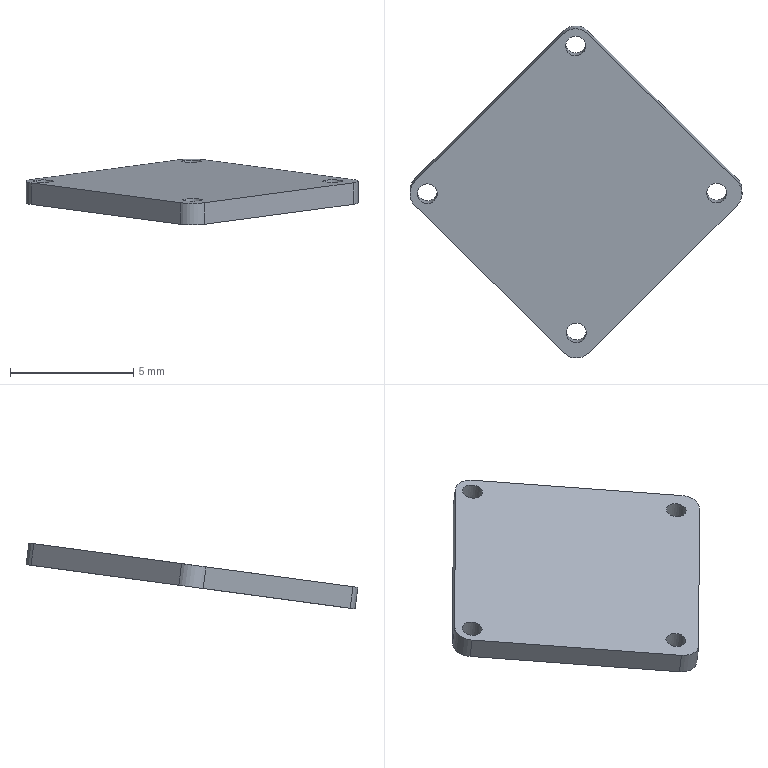Part | SolidWorks | features SplitBody 1 | 1 solid | 18 faces | box 13.455 x 13.452 x 2.67 mm | volume 84.523 mm3 | cylinder 12 | plane 6 | commonest cylinder face diameters 0.81 x8 1.408 x4
STEP:
#1=CARTESIAN_POINT('',(579.092,436.156,-315.844));
#2=VERTEX_POINT('',#1);
#3=CARTESIAN_POINT('',(579.666,435.59,-315.921));
#4=VERTEX_POINT('',#3);
#5=CARTESIAN_POINT('',(579.379,435.873,-315.882));
#6=DIRECTION('',(0.,-0.1337,0.991));
#7=DIRECTION('',(0.7089,-0.6989,-0.09427));
#8=AXIS2_PLACEMENT_3D('',#5,#6,#7);
#9=CIRCLE('',#8,0.4048);
#10=EDGE_CURVE('',#2,#4,#9,.T.);
#11=ORIENTED_EDGE('',*,*,#10,.T.);
#12=CARTESIAN_POINT('',(579.666,435.708,-316.793));
#13=VERTEX_POINT('',#12);
#14=CARTESIAN_POINT('',(579.666,435.59,-315.921));
#15=DIRECTION('',(0.,0.1337,-0.991));
#16=VECTOR('',#15,1000.);
#17=LINE('',#14,#16);
#18=EDGE_CURVE('',#4,#13,#17,.T.);
#19=ORIENTED_EDGE('',*,*,#18,.T.);
#20=CARTESIAN_POINT('',(579.092,436.274,-316.716));
#21=VERTEX_POINT('',#20);
#22=CARTESIAN_POINT('',(579.379,435.991,-316.754));
#23=DIRECTION('',(0.,-0.1337,0.991));
#24=DIRECTION('',(0.7089,-0.6989,-0.09427));
#25=AXIS2_PLACEMENT_3D('',#22,#23,#24);
#26=CIRCLE('',#25,0.4048);
#27=EDGE_CURVE('',#21,#13,#26,.T.);
#28=ORIENTED_EDGE('',*,*,#27,.F.);
#29=CARTESIAN_POINT('',(579.092,436.156,-315.844));
#30=DIRECTION('',(0.,0.1337,-0.991));
#31=VECTOR('',#30,1000.);
#32=LINE('',#29,#31);
#33=EDGE_CURVE('',#2,#21,#32,.T.);
#34=ORIENTED_EDGE('',*,*,#33,.F.);
#35=EDGE_LOOP('',(#11,#19,#28,#34));
#36=FACE_OUTER_BOUND('',#35,.T.);
#37=CARTESIAN_POINT('',(579.379,435.873,-315.882));
#38=DIRECTION('',(0.,0.1337,-0.991));
#39=DIRECTION('',(-0.7089,0.6989,0.09427));
#40=AXIS2_PLACEMENT_3D('',#37,#38,#39);
#41=CYLINDRICAL_SURFACE('',#40,0.4048);
#42=ADVANCED_FACE('',(#36),#41,.F.);
#43=CARTESIAN_POINT('',(573.053,441.789,-315.084));
#44=VERTEX_POINT('',#43);
#45=CARTESIAN_POINT('',(573.627,441.224,-315.161));
#46=VERTEX_POINT('',#45);
#47=CARTESIAN_POINT('',(573.34,441.507,-315.123));
#48=DIRECTION('',(0.,-0.1337,0.991));
#49=DIRECTION('',(0.7089,-0.6989,-0.09427));
#50=AXIS2_PLACEMENT_3D('',#47,#48,#49);
#51=CIRCLE('',#50,0.4048);
#52=EDGE_CURVE('',#44,#46,#51,.T.);
#53=ORIENTED_EDGE('',*,*,#52,.T.);
#54=CARTESIAN_POINT('',(573.627,441.341,-316.033));
#55=VERTEX_POINT('',#54);
#56=CARTESIAN_POINT('',(573.627,441.224,-315.161));
#57=DIRECTION('',(0.,0.1337,-0.991));
#58=VECTOR('',#57,1000.);
#59=LINE('',#56,#58);
#60=EDGE_CURVE('',#46,#55,#59,.T.);
#61=ORIENTED_EDGE('',*,*,#60,.T.);
#62=CARTESIAN_POINT('',(573.053,441.907,-315.957));
#63=VERTEX_POINT('',#62);
#64=CARTESIAN_POINT('',(573.34,441.624,-315.995));
#65=DIRECTION('',(0.,-0.1337,0.991));
#66=DIRECTION('',(0.7089,-0.6989,-0.09427));
#67=AXIS2_PLACEMENT_3D('',#64,#65,#66);
#68=CIRCLE('',#67,0.4048);
#69=EDGE_CURVE('',#63,#55,#68,.T.);
#70=ORIENTED_EDGE('',*,*,#69,.F.);
#71=CARTESIAN_POINT('',(573.053,441.789,-315.084));
#72=DIRECTION('',(0.,0.1337,-0.991));
#73=VECTOR('',#72,1000.);
#74=LINE('',#71,#73);
#75=EDGE_CURVE('',#44,#63,#74,.T.);
#76=ORIENTED_EDGE('',*,*,#75,.F.);
#77=EDGE_LOOP('',(#53,#61,#70,#76));
#78=FACE_OUTER_BOUND('',#77,.T.);
#79=CARTESIAN_POINT('',(573.34,441.507,-315.123));
#80=DIRECTION('',(0.,0.1337,-0.991));
#81=DIRECTION('',(-0.7089,0.6989,0.09427));
#82=AXIS2_PLACEMENT_3D('',#79,#80,#81);
#83=CYLINDRICAL_SURFACE('',#82,0.4048);
#84=ADVANCED_FACE('',(#78),#83,.F.);
#85=CARTESIAN_POINT('',(584.777,441.82,-315.08));
#86=VERTEX_POINT('',#85);
#87=CARTESIAN_POINT('',(585.351,441.254,-315.157));
#88=VERTEX_POINT('',#87);
#89=CARTESIAN_POINT('',(585.064,441.537,-315.119));
#90=DIRECTION('',(0.,-0.1337,0.991));
#91=DIRECTION('',(0.7089,-0.6989,-0.09427));
#92=AXIS2_PLACEMENT_3D('',#89,#90,#91);
#93=CIRCLE('',#92,0.4048);
#94=EDGE_CURVE('',#86,#88,#93,.T.);
#95=ORIENTED_EDGE('',*,*,#94,.T.);
#96=CARTESIAN_POINT('',(585.351,441.372,-316.029));
#97=VERTEX_POINT('',#96);
#98=CARTESIAN_POINT('',(585.351,441.254,-315.157));
#99=DIRECTION('',(0.,0.1337,-0.991));
#100=VECTOR('',#99,1000.);
#101=LINE('',#98,#100);
#102=EDGE_CURVE('',#88,#97,#101,.T.);
#103=ORIENTED_EDGE('',*,*,#102,.T.);
#104=CARTESIAN_POINT('',(584.777,441.937,-315.952));
#105=VERTEX_POINT('',#104);
#106=CARTESIAN_POINT('',(585.064,441.654,-315.991));
#107=DIRECTION('',(0.,-0.1337,0.991));
#108=DIRECTION('',(0.7089,-0.6989,-0.09427));
#109=AXIS2_PLACEMENT_3D('',#106,#107,#108);
#110=CIRCLE('',#109,0.4048);
#111=EDGE_CURVE('',#105,#97,#110,.T.);
#112=ORIENTED_EDGE('',*,*,#111,.F.);
#113=CARTESIAN_POINT('',(584.777,441.82,-315.08));
#114=DIRECTION('',(0.,0.1337,-0.991));
#115=VECTOR('',#114,1000.);
#116=LINE('',#113,#115);
#117=EDGE_CURVE('',#86,#105,#116,.T.);
#118=ORIENTED_EDGE('',*,*,#117,.F.);
#119=EDGE_LOOP('',(#95,#103,#112,#118));
#120=FACE_OUTER_BOUND('',#119,.T.);
#121=CARTESIAN_POINT('',(585.064,441.537,-315.119));
#122=DIRECTION('',(0.,0.1337,-0.991));
#123=DIRECTION('',(-0.7089,0.6989,0.09427));
#124=AXIS2_PLACEMENT_3D('',#121,#122,#123);
#125=CYLINDRICAL_SURFACE('',#124,0.4048);
#126=ADVANCED_FACE('',(#120),#125,.F.);
#127=CARTESIAN_POINT('',(579.061,447.774,-314.277));
#128=VERTEX_POINT('',#127);
#129=CARTESIAN_POINT('',(579.635,447.209,-314.354));
#130=VERTEX_POINT('',#129);
#131=CARTESIAN_POINT('',(579.348,447.491,-314.315));
#132=DIRECTION('',(0.,-0.1337,0.991));
#133=DIRECTION('',(0.7089,-0.6989,-0.09427));
#134=AXIS2_PLACEMENT_3D('',#131,#132,#133);
#135=CIRCLE('',#134,0.4048);
#136=EDGE_CURVE('',#128,#130,#135,.T.);
#137=ORIENTED_EDGE('',*,*,#136,.T.);
#138=CARTESIAN_POINT('',(579.635,447.326,-315.226));
#139=VERTEX_POINT('',#138);
#140=CARTESIAN_POINT('',(579.635,447.209,-314.354));
#141=DIRECTION('',(0.,0.1337,-0.991));
#142=VECTOR('',#141,1000.);
#143=LINE('',#140,#142);
#144=EDGE_CURVE('',#130,#139,#143,.T.);
#145=ORIENTED_EDGE('',*,*,#144,.T.);
#146=CARTESIAN_POINT('',(579.061,447.892,-315.149));
#147=VERTEX_POINT('',#146);
#148=CARTESIAN_POINT('',(579.348,447.609,-315.188));
#149=DIRECTION('',(0.,-0.1337,0.991));
#150=DIRECTION('',(0.7089,-0.6989,-0.09427));
#151=AXIS2_PLACEMENT_3D('',#148,#149,#150);
#152=CIRCLE('',#151,0.4048);
#153=EDGE_CURVE('',#147,#139,#152,.T.);
#154=ORIENTED_EDGE('',*,*,#153,.F.);
#155=CARTESIAN_POINT('',(579.061,447.774,-314.277));
#156=DIRECTION('',(0.,0.1337,-0.991));
#157=VECTOR('',#156,1000.);
#158=LINE('',#155,#157);
#159=EDGE_CURVE('',#128,#147,#158,.T.);
#160=ORIENTED_EDGE('',*,*,#159,.F.);
#161=EDGE_LOOP('',(#137,#145,#154,#160));
#162=FACE_OUTER_BOUND('',#161,.T.);
#163=CARTESIAN_POINT('',(579.348,447.491,-314.315));
#164=DIRECTION('',(0.,0.1337,-0.991));
#165=DIRECTION('',(-0.7089,0.6989,0.09427));
#166=AXIS2_PLACEMENT_3D('',#163,#164,#165);
#167=CYLINDRICAL_SURFACE('',#166,0.4048);
#168=ADVANCED_FACE('',(#162),#167,.F.);
#169=ORIENTED_EDGE('',*,*,#52,.F.);
#170=CARTESIAN_POINT('',(573.34,441.507,-315.123));
#171=DIRECTION('',(0.,-0.1337,0.991));
#172=DIRECTION('',(0.7089,-0.6989,-0.09427));
#173=AXIS2_PLACEMENT_3D('',#170,#171,#172);
#174=CIRCLE('',#173,0.4048);
#175=EDGE_CURVE('',#46,#44,#174,.T.);
#176=ORIENTED_EDGE('',*,*,#175,.F.);
#177=EDGE_LOOP('',(#169,#176));
#178=FACE_BOUND('',#177,.T.);
#179=ORIENTED_EDGE('',*,*,#136,.F.);
#180=CARTESIAN_POINT('',(579.348,447.491,-314.315));
#181=DIRECTION('',(0.,-0.1337,0.991));
#182=DIRECTION('',(0.7089,-0.6989,-0.09427));
#183=AXIS2_PLACEMENT_3D('',#180,#181,#182);
#184=CIRCLE('',#183,0.4048);
#185=EDGE_CURVE('',#130,#128,#184,.T.);
#186=ORIENTED_EDGE('',*,*,#185,.F.);
#187=EDGE_LOOP('',(#179,#186));
#188=FACE_BOUND('',#187,.T.);
#189=CARTESIAN_POINT('',(572.841,441.999,-315.056));
#190=VERTEX_POINT('',#189);
#191=CARTESIAN_POINT('',(572.844,441.012,-315.189));
#192=VERTEX_POINT('',#191);
#193=CARTESIAN_POINT('',(573.34,441.507,-315.123));
#194=DIRECTION('',(0.,-0.1337,0.991));
#195=DIRECTION('',(-0.7089,0.6989,0.09427));
#196=AXIS2_PLACEMENT_3D('',#193,#194,#195);
#197=CIRCLE('',#196,0.704);
#198=EDGE_CURVE('',#190,#192,#197,.T.);
#199=ORIENTED_EDGE('',*,*,#198,.T.);
#200=CARTESIAN_POINT('',(578.883,435.058,-315.992));
#201=VERTEX_POINT('',#200);
#202=CARTESIAN_POINT('',(572.844,441.012,-315.189));
#203=DIRECTION('',(0.7089,-0.6989,-0.09427));
#204=VECTOR('',#203,1000.);
#205=LINE('',#202,#204);
#206=EDGE_CURVE('',#192,#201,#205,.T.);
#207=ORIENTED_EDGE('',*,*,#206,.T.);
#208=CARTESIAN_POINT('',(579.879,435.061,-315.992));
#209=VERTEX_POINT('',#208);
#210=CARTESIAN_POINT('',(579.379,435.553,-315.926));
#211=DIRECTION('',(0.,-0.1337,0.991));
#212=DIRECTION('',(0.7089,-0.6989,-0.09427));
#213=AXIS2_PLACEMENT_3D('',#210,#211,#212);
#214=CIRCLE('',#213,0.704);
#215=EDGE_CURVE('',#201,#209,#214,.T.);
#216=ORIENTED_EDGE('',*,*,#215,.T.);
#217=CARTESIAN_POINT('',(585.886,441.046,-315.185));
#218=VERTEX_POINT('',#217);
#219=CARTESIAN_POINT('',(579.879,435.061,-315.992));
#220=DIRECTION('',(0.7053,0.7026,0.09476));
#221=VECTOR('',#220,1000.);
#222=LINE('',#219,#221);
#223=EDGE_CURVE('',#209,#218,#222,.T.);
#224=ORIENTED_EDGE('',*,*,#223,.T.);
#225=CARTESIAN_POINT('',(585.884,442.032,-315.052));
#226=VERTEX_POINT('',#225);
#227=CARTESIAN_POINT('',(585.387,441.538,-315.118));
#228=DIRECTION('',(0.,-0.1337,0.991));
#229=DIRECTION('',(-0.7089,0.6989,0.09427));
#230=AXIS2_PLACEMENT_3D('',#227,#228,#229);
#231=CIRCLE('',#230,0.704);
#232=EDGE_CURVE('',#218,#226,#231,.T.);
#233=ORIENTED_EDGE('',*,*,#232,.T.);
#234=CARTESIAN_POINT('',(579.845,447.986,-314.249));
#235=VERTEX_POINT('',#234);
#236=CARTESIAN_POINT('',(579.845,447.986,-314.249));
#237=DIRECTION('',(-0.7089,0.6989,0.09427));
#238=VECTOR('',#237,1000.);
#239=LINE('',#236,#238);
#240=EDGE_CURVE('',#226,#235,#239,.T.);
#241=ORIENTED_EDGE('',*,*,#240,.T.);
#242=CARTESIAN_POINT('',(578.849,447.984,-314.249));
#243=VERTEX_POINT('',#242);
#244=CARTESIAN_POINT('',(579.348,447.491,-314.315));
#245=DIRECTION('',(0.,-0.1337,0.991));
#246=DIRECTION('',(-0.7089,0.6989,0.09427));
#247=AXIS2_PLACEMENT_3D('',#244,#245,#246);
#248=CIRCLE('',#247,0.704);
#249=EDGE_CURVE('',#235,#243,#248,.T.);
#250=ORIENTED_EDGE('',*,*,#249,.T.);
#251=CARTESIAN_POINT('',(572.841,441.999,-315.056));
#252=DIRECTION('',(-0.7053,-0.7026,-0.09476));
#253=VECTOR('',#252,1000.);
#254=LINE('',#251,#253);
#255=EDGE_CURVE('',#243,#190,#254,.T.);
#256=ORIENTED_EDGE('',*,*,#255,.T.);
#257=EDGE_LOOP('',(#199,#207,#216,#224,#233,#241,#250,#256));
#258=FACE_OUTER_BOUND('',#257,.T.);
#259=ORIENTED_EDGE('',*,*,#94,.F.);
#260=CARTESIAN_POINT('',(585.064,441.537,-315.119));
#261=DIRECTION('',(0.,-0.1337,0.991));
#262=DIRECTION('',(0.7089,-0.6989,-0.09427));
#263=AXIS2_PLACEMENT_3D('',#260,#261,#262);
#264=CIRCLE('',#263,0.4048);
#265=EDGE_CURVE('',#88,#86,#264,.T.);
#266=ORIENTED_EDGE('',*,*,#265,.F.);
#267=EDGE_LOOP('',(#259,#266));
#268=FACE_BOUND('',#267,.T.);
#269=ORIENTED_EDGE('',*,*,#10,.F.);
#270=CARTESIAN_POINT('',(579.379,435.873,-315.882));
#271=DIRECTION('',(0.,-0.1337,0.991));
#272=DIRECTION('',(0.7089,-0.6989,-0.09427));
#273=AXIS2_PLACEMENT_3D('',#270,#271,#272);
#274=CIRCLE('',#273,0.4048);
#275=EDGE_CURVE('',#4,#2,#274,.T.);
#276=ORIENTED_EDGE('',*,*,#275,.F.);
#277=EDGE_LOOP('',(#269,#276));
#278=FACE_BOUND('',#277,.T.);
#279=CARTESIAN_POINT('',(573.34,441.507,-315.123));
#280=DIRECTION('',(0.,0.1337,-0.991));
#281=DIRECTION('',(-0.7089,0.6989,0.09427));
#282=AXIS2_PLACEMENT_3D('',#279,#280,#281);
#283=PLANE('',#282);
#284=ADVANCED_FACE('',(#178,#188,#258,#268,#278),#283,.F.);
#285=ORIENTED_EDGE('',*,*,#69,.T.);
#286=CARTESIAN_POINT('',(573.34,441.624,-315.995));
#287=DIRECTION('',(0.,-0.1337,0.991));
#288=DIRECTION('',(0.7089,-0.6989,-0.09427));
#289=AXIS2_PLACEMENT_3D('',#286,#287,#288);
#290=CIRCLE('',#289,0.4048);
#291=EDGE_CURVE('',#55,#63,#290,.T.);
#292=ORIENTED_EDGE('',*,*,#291,.T.);
#293=EDGE_LOOP('',(#285,#292));
#294=FACE_BOUND('',#293,.T.);
#295=ORIENTED_EDGE('',*,*,#153,.T.);
#296=CARTESIAN_POINT('',(579.348,447.609,-315.188));
#297=DIRECTION('',(0.,-0.1337,0.991));
#298=DIRECTION('',(0.7089,-0.6989,-0.09427));
#299=AXIS2_PLACEMENT_3D('',#296,#297,#298);
#300=CIRCLE('',#299,0.4048);
#301=EDGE_CURVE('',#139,#147,#300,.T.);
#302=ORIENTED_EDGE('',*,*,#301,.T.);
#303=EDGE_LOOP('',(#295,#302));
#304=FACE_BOUND('',#303,.T.);
#305=CARTESIAN_POINT('',(572.841,442.116,-315.928));
#306=VERTEX_POINT('',#305);
#307=CARTESIAN_POINT('',(572.844,441.13,-316.061));
#308=VERTEX_POINT('',#307);
#309=CARTESIAN_POINT('',(573.34,441.624,-315.995));
#310=DIRECTION('',(0.,-0.1337,0.991));
#311=DIRECTION('',(-0.7089,0.6989,0.09427));
#312=AXIS2_PLACEMENT_3D('',#309,#310,#311);
#313=CIRCLE('',#312,0.704);
#314=EDGE_CURVE('',#306,#308,#313,.T.);
#315=ORIENTED_EDGE('',*,*,#314,.F.);
#316=CARTESIAN_POINT('',(578.849,448.101,-315.121));
#317=VERTEX_POINT('',#316);
#318=CARTESIAN_POINT('',(572.841,442.116,-315.928));
#319=DIRECTION('',(-0.7053,-0.7026,-0.09476));
#320=VECTOR('',#319,1000.);
#321=LINE('',#318,#320);
#322=EDGE_CURVE('',#317,#306,#321,.T.);
#323=ORIENTED_EDGE('',*,*,#322,.F.);
#324=CARTESIAN_POINT('',(579.845,448.104,-315.121));
#325=VERTEX_POINT('',#324);
#326=CARTESIAN_POINT('',(579.348,447.609,-315.188));
#327=DIRECTION('',(0.,-0.1337,0.991));
#328=DIRECTION('',(-0.7089,0.6989,0.09427));
#329=AXIS2_PLACEMENT_3D('',#326,#327,#328);
#330=CIRCLE('',#329,0.704);
#331=EDGE_CURVE('',#325,#317,#330,.T.);
#332=ORIENTED_EDGE('',*,*,#331,.F.);
#333=CARTESIAN_POINT('',(585.884,442.15,-315.924));
#334=VERTEX_POINT('',#333);
#335=CARTESIAN_POINT('',(579.845,448.104,-315.121));
#336=DIRECTION('',(-0.7089,0.6989,0.09427));
#337=VECTOR('',#336,1000.);
#338=LINE('',#335,#337);
#339=EDGE_CURVE('',#334,#325,#338,.T.);
#340=ORIENTED_EDGE('',*,*,#339,.F.);
#341=CARTESIAN_POINT('',(585.886,441.163,-316.057));
#342=VERTEX_POINT('',#341);
#343=CARTESIAN_POINT('',(585.387,441.655,-315.991));
#344=DIRECTION('',(0.,-0.1337,0.991));
#345=DIRECTION('',(-0.7089,0.6989,0.09427));
#346=AXIS2_PLACEMENT_3D('',#343,#344,#345);
#347=CIRCLE('',#346,0.704);
#348=EDGE_CURVE('',#342,#334,#347,.T.);
#349=ORIENTED_EDGE('',*,*,#348,.F.);
#350=CARTESIAN_POINT('',(579.879,435.178,-316.864));
#351=VERTEX_POINT('',#350);
#352=CARTESIAN_POINT('',(579.879,435.178,-316.864));
#353=DIRECTION('',(0.7053,0.7026,0.09476));
#354=VECTOR('',#353,1000.);
#355=LINE('',#352,#354);
#356=EDGE_CURVE('',#351,#342,#355,.T.);
#357=ORIENTED_EDGE('',*,*,#356,.F.);
#358=CARTESIAN_POINT('',(578.883,435.176,-316.864));
#359=VERTEX_POINT('',#358);
#360=CARTESIAN_POINT('',(579.379,435.67,-316.798));
#361=DIRECTION('',(0.,-0.1337,0.991));
#362=DIRECTION('',(0.7089,-0.6989,-0.09427));
#363=AXIS2_PLACEMENT_3D('',#360,#361,#362);
#364=CIRCLE('',#363,0.704);
#365=EDGE_CURVE('',#359,#351,#364,.T.);
#366=ORIENTED_EDGE('',*,*,#365,.F.);
#367=CARTESIAN_POINT('',(572.844,441.13,-316.061));
#368=DIRECTION('',(0.7089,-0.6989,-0.09427));
#369=VECTOR('',#368,1000.);
#370=LINE('',#367,#369);
#371=EDGE_CURVE('',#308,#359,#370,.T.);
#372=ORIENTED_EDGE('',*,*,#371,.F.);
#373=EDGE_LOOP('',(#315,#323,#332,#340,#349,#357,#366,#372));
#374=FACE_OUTER_BOUND('',#373,.T.);
#375=ORIENTED_EDGE('',*,*,#111,.T.);
#376=CARTESIAN_POINT('',(585.064,441.654,-315.991));
#377=DIRECTION('',(0.,-0.1337,0.991));
#378=DIRECTION('',(0.7089,-0.6989,-0.09427));
#379=AXIS2_PLACEMENT_3D('',#376,#377,#378);
#380=CIRCLE('',#379,0.4048);
#381=EDGE_CURVE('',#97,#105,#380,.T.);
#382=ORIENTED_EDGE('',*,*,#381,.T.);
#383=EDGE_LOOP('',(#375,#382));
#384=FACE_BOUND('',#383,.T.);
#385=ORIENTED_EDGE('',*,*,#27,.T.);
#386=CARTESIAN_POINT('',(579.379,435.991,-316.754));
#387=DIRECTION('',(0.,-0.1337,0.991));
#388=DIRECTION('',(0.7089,-0.6989,-0.09427));
#389=AXIS2_PLACEMENT_3D('',#386,#387,#388);
#390=CIRCLE('',#389,0.4048);
#391=EDGE_CURVE('',#13,#21,#390,.T.);
#392=ORIENTED_EDGE('',*,*,#391,.T.);
#393=EDGE_LOOP('',(#385,#392));
#394=FACE_BOUND('',#393,.T.);
#395=CARTESIAN_POINT('',(573.34,441.624,-315.995));
#396=DIRECTION('',(0.,0.1337,-0.991));
#397=DIRECTION('',(-0.7089,0.6989,0.09427));
#398=AXIS2_PLACEMENT_3D('',#395,#396,#397);
#399=PLANE('',#398);
#400=ADVANCED_FACE('',(#294,#304,#374,#384,#394),#399,.T.);
#401=ORIENTED_EDGE('',*,*,#314,.T.);
#402=CARTESIAN_POINT('',(572.844,441.012,-315.189));
#403=DIRECTION('',(0.,0.1337,-0.991));
#404=VECTOR('',#403,1000.);
#405=LINE('',#402,#404);
#406=EDGE_CURVE('',#192,#308,#405,.T.);
#407=ORIENTED_EDGE('',*,*,#406,.F.);
#408=ORIENTED_EDGE('',*,*,#198,.F.);
#409=CARTESIAN_POINT('',(572.841,441.999,-315.056));
#410=DIRECTION('',(0.,0.1337,-0.991));
#411=VECTOR('',#410,1000.);
#412=LINE('',#409,#411);
#413=EDGE_CURVE('',#190,#306,#412,.T.);
#414=ORIENTED_EDGE('',*,*,#413,.T.);
#415=EDGE_LOOP('',(#401,#407,#408,#414));
#416=FACE_OUTER_BOUND('',#415,.T.);
#417=CARTESIAN_POINT('',(573.34,441.507,-315.123));
#418=DIRECTION('',(0.,0.1337,-0.991));
#419=DIRECTION('',(-0.7089,0.6989,0.09427));
#420=AXIS2_PLACEMENT_3D('',#417,#418,#419);
#421=CYLINDRICAL_SURFACE('',#420,0.704);
#422=ADVANCED_FACE('',(#416),#421,.T.);
#423=ORIENTED_EDGE('',*,*,#371,.T.);
#424=CARTESIAN_POINT('',(578.883,435.058,-315.992));
#425=DIRECTION('',(0.,0.1337,-0.991));
#426=VECTOR('',#425,1000.);
#427=LINE('',#424,#426);
#428=EDGE_CURVE('',#201,#359,#427,.T.);
#429=ORIENTED_EDGE('',*,*,#428,.F.);
#430=ORIENTED_EDGE('',*,*,#206,.F.);
#431=ORIENTED_EDGE('',*,*,#406,.T.);
#432=EDGE_LOOP('',(#423,#429,#430,#431));
#433=FACE_OUTER_BOUND('',#432,.T.);
#434=CARTESIAN_POINT('',(572.844,441.012,-315.189));
#435=DIRECTION('',(0.7053,0.7026,0.09476));
#436=DIRECTION('',(0.,-0.1337,0.991));
#437=AXIS2_PLACEMENT_3D('',#434,#435,#436);
#438=PLANE('',#437);
#439=ADVANCED_FACE('',(#433),#438,.F.);
#440=ORIENTED_EDGE('',*,*,#365,.T.);
#441=CARTESIAN_POINT('',(579.879,435.061,-315.992));
#442=DIRECTION('',(0.,0.1337,-0.991));
#443=VECTOR('',#442,1000.);
#444=LINE('',#441,#443);
#445=EDGE_CURVE('',#209,#351,#444,.T.);
#446=ORIENTED_EDGE('',*,*,#445,.F.);
#447=ORIENTED_EDGE('',*,*,#215,.F.);
#448=ORIENTED_EDGE('',*,*,#428,.T.);
#449=EDGE_LOOP('',(#440,#446,#447,#448));
#450=FACE_OUTER_BOUND('',#449,.T.);
#451=CARTESIAN_POINT('',(579.379,435.553,-315.926));
#452=DIRECTION('',(0.,0.1337,-0.991));
#453=DIRECTION('',(-0.7089,0.6989,0.09427));
#454=AXIS2_PLACEMENT_3D('',#451,#452,#453);
#455=CYLINDRICAL_SURFACE('',#454,0.704);
#456=ADVANCED_FACE('',(#450),#455,.T.);
#457=ORIENTED_EDGE('',*,*,#356,.T.);
#458=CARTESIAN_POINT('',(585.886,441.046,-315.185));
#459=DIRECTION('',(0.,0.1337,-0.991));
#460=VECTOR('',#459,1000.);
#461=LINE('',#458,#460);
#462=EDGE_CURVE('',#218,#342,#461,.T.);
#463=ORIENTED_EDGE('',*,*,#462,.F.);
#464=ORIENTED_EDGE('',*,*,#223,.F.);
#465=ORIENTED_EDGE('',*,*,#445,.T.);
#466=EDGE_LOOP('',(#457,#463,#464,#465));
#467=FACE_OUTER_BOUND('',#466,.T.);
#468=CARTESIAN_POINT('',(579.879,435.061,-315.992));
#469=DIRECTION('',(-0.7089,0.6989,0.09427));
#470=DIRECTION('',(0.,-0.1337,0.991));
#471=AXIS2_PLACEMENT_3D('',#468,#469,#470);
#472=PLANE('',#471);
#473=ADVANCED_FACE('',(#467),#472,.F.);
#474=ORIENTED_EDGE('',*,*,#348,.T.);
#475=CARTESIAN_POINT('',(585.884,442.032,-315.052));
#476=DIRECTION('',(0.,0.1337,-0.991));
#477=VECTOR('',#476,1000.);
#478=LINE('',#475,#477);
#479=EDGE_CURVE('',#226,#334,#478,.T.);
#480=ORIENTED_EDGE('',*,*,#479,.F.);
#481=ORIENTED_EDGE('',*,*,#232,.F.);
#482=ORIENTED_EDGE('',*,*,#462,.T.);
#483=EDGE_LOOP('',(#474,#480,#481,#482));
#484=FACE_OUTER_BOUND('',#483,.T.);
#485=CARTESIAN_POINT('',(585.387,441.538,-315.118));
#486=DIRECTION('',(0.,0.1337,-0.991));
#487=DIRECTION('',(-0.7089,0.6989,0.09427));
#488=AXIS2_PLACEMENT_3D('',#485,#486,#487);
#489=CYLINDRICAL_SURFACE('',#488,0.704);
#490=ADVANCED_FACE('',(#484),#489,.T.);
#491=ORIENTED_EDGE('',*,*,#339,.T.);
#492=CARTESIAN_POINT('',(579.845,447.986,-314.249));
#493=DIRECTION('',(0.,0.1337,-0.991));
#494=VECTOR('',#493,1000.);
#495=LINE('',#492,#494);
#496=EDGE_CURVE('',#235,#325,#495,.T.);
#497=ORIENTED_EDGE('',*,*,#496,.F.);
#498=ORIENTED_EDGE('',*,*,#240,.F.);
#499=ORIENTED_EDGE('',*,*,#479,.T.);
#500=EDGE_LOOP('',(#491,#497,#498,#499));
#501=FACE_OUTER_BOUND('',#500,.T.);
#502=CARTESIAN_POINT('',(579.845,447.986,-314.249));
#503=DIRECTION('',(-0.7053,-0.7026,-0.09476));
#504=DIRECTION('',(0.,0.1337,-0.991));
#505=AXIS2_PLACEMENT_3D('',#502,#503,#504);
#506=PLANE('',#505);
#507=ADVANCED_FACE('',(#501),#506,.F.);
#508=ORIENTED_EDGE('',*,*,#331,.T.);
#509=CARTESIAN_POINT('',(578.849,447.984,-314.249));
#510=DIRECTION('',(0.,0.1337,-0.991));
#511=VECTOR('',#510,1000.);
#512=LINE('',#509,#511);
#513=EDGE_CURVE('',#243,#317,#512,.T.);
#514=ORIENTED_EDGE('',*,*,#513,.F.);
#515=ORIENTED_EDGE('',*,*,#249,.F.);
#516=ORIENTED_EDGE('',*,*,#496,.T.);
#517=EDGE_LOOP('',(#508,#514,#515,#516));
#518=FACE_OUTER_BOUND('',#517,.T.);
#519=CARTESIAN_POINT('',(579.348,447.491,-314.315));
#520=DIRECTION('',(0.,0.1337,-0.991));
#521=DIRECTION('',(-0.7089,0.6989,0.09427));
#522=AXIS2_PLACEMENT_3D('',#519,#520,#521);
#523=CYLINDRICAL_SURFACE('',#522,0.704);
#524=ADVANCED_FACE('',(#518),#523,.T.);
#525=ORIENTED_EDGE('',*,*,#322,.T.);
#526=ORIENTED_EDGE('',*,*,#413,.F.);
#527=ORIENTED_EDGE('',*,*,#255,.F.);
#528=ORIENTED_EDGE('',*,*,#513,.T.);
#529=EDGE_LOOP('',(#525,#526,#527,#528));
#530=FACE_OUTER_BOUND('',#529,.T.);
#531=CARTESIAN_POINT('',(572.841,441.999,-315.056));
#532=DIRECTION('',(0.7089,-0.6989,-0.09427));
#533=DIRECTION('',(0.,0.1337,-0.991));
#534=AXIS2_PLACEMENT_3D('',#531,#532,#533);
#535=PLANE('',#534);
#536=ADVANCED_FACE('',(#530),#535,.F.);
#537=ORIENTED_EDGE('',*,*,#144,.F.);
#538=ORIENTED_EDGE('',*,*,#185,.T.);
#539=ORIENTED_EDGE('',*,*,#159,.T.);
#540=ORIENTED_EDGE('',*,*,#301,.F.);
#541=EDGE_LOOP('',(#537,#538,#539,#540));
#542=FACE_OUTER_BOUND('',#541,.T.);
#543=CARTESIAN_POINT('',(579.348,447.491,-314.315));
#544=DIRECTION('',(0.,0.1337,-0.991));
#545=DIRECTION('',(-0.7089,0.6989,0.09427));
#546=AXIS2_PLACEMENT_3D('',#543,#544,#545);
#547=CYLINDRICAL_SURFACE('',#546,0.4048);
#548=ADVANCED_FACE('',(#542),#547,.F.);
#549=ORIENTED_EDGE('',*,*,#102,.F.);
#550=ORIENTED_EDGE('',*,*,#265,.T.);
#551=ORIENTED_EDGE('',*,*,#117,.T.);
#552=ORIENTED_EDGE('',*,*,#381,.F.);
#553=EDGE_LOOP('',(#549,#550,#551,#552));
#554=FACE_OUTER_BOUND('',#553,.T.);
#555=CARTESIAN_POINT('',(585.064,441.537,-315.119));
#556=DIRECTION('',(0.,0.1337,-0.991));
#557=DIRECTION('',(-0.7089,0.6989,0.09427));
#558=AXIS2_PLACEMENT_3D('',#555,#556,#557);
#559=CYLINDRICAL_SURFACE('',#558,0.4048);
#560=ADVANCED_FACE('',(#554),#559,.F.);
#561=ORIENTED_EDGE('',*,*,#60,.F.);
#562=ORIENTED_EDGE('',*,*,#175,.T.);
#563=ORIENTED_EDGE('',*,*,#75,.T.);
#564=ORIENTED_EDGE('',*,*,#291,.F.);
#565=EDGE_LOOP('',(#561,#562,#563,#564));
#566=FACE_OUTER_BOUND('',#565,.T.);
#567=CARTESIAN_POINT('',(573.34,441.507,-315.123));
#568=DIRECTION('',(0.,0.1337,-0.991));
#569=DIRECTION('',(-0.7089,0.6989,0.09427));
#570=AXIS2_PLACEMENT_3D('',#567,#568,#569);
#571=CYLINDRICAL_SURFACE('',#570,0.4048);
#572=ADVANCED_FACE('',(#566),#571,.F.);
#573=ORIENTED_EDGE('',*,*,#18,.F.);
#574=ORIENTED_EDGE('',*,*,#275,.T.);
#575=ORIENTED_EDGE('',*,*,#33,.T.);
#576=ORIENTED_EDGE('',*,*,#391,.F.);
#577=EDGE_LOOP('',(#573,#574,#575,#576));
#578=FACE_OUTER_BOUND('',#577,.T.);
#579=CARTESIAN_POINT('',(579.379,435.873,-315.882));
#580=DIRECTION('',(0.,0.1337,-0.991));
#581=DIRECTION('',(-0.7089,0.6989,0.09427));
#582=AXIS2_PLACEMENT_3D('',#579,#580,#581);
#583=CYLINDRICAL_SURFACE('',#582,0.4048);
#584=ADVANCED_FACE('',(#578),#583,.F.);
#585=CLOSED_SHELL('',(#42,#84,#126,#168,#284,#400,#422,#439,#456,#473,#490,#507,#524,#536,#548,#560,#572,#584));
#586=MANIFOLD_SOLID_BREP('',#585);
#587=CARTESIAN_POINT('',(0.,0.,0.));
#588=DIRECTION('',(0.,0.,1.));
#589=DIRECTION('',(1.,0.,0.));
#590=AXIS2_PLACEMENT_3D('',#587,#588,#589);
#591=(LENGTH_UNIT()NAMED_UNIT(*)SI_UNIT(.MILLI.,.METRE.));
#592=UNCERTAINTY_MEASURE_WITH_UNIT(LENGTH_MEASURE(0.00001),#591,'','');
#593=(NAMED_UNIT(*)PLANE_ANGLE_UNIT()SI_UNIT($,.RADIAN.));
#594=(NAMED_UNIT(*)SI_UNIT($,.STERADIAN.)SOLID_ANGLE_UNIT());
#595=(GEOMETRIC_REPRESENTATION_CONTEXT(3)GLOBAL_UNCERTAINTY_ASSIGNED_CONTEXT((#592))GLOBAL_UNIT_ASSIGNED_CONTEXT((#591,#593,#594))REPRESENTATION_CONTEXT('',''));
#596=ADVANCED_BREP_SHAPE_REPRESENTATION('',(#586,#590),#595);